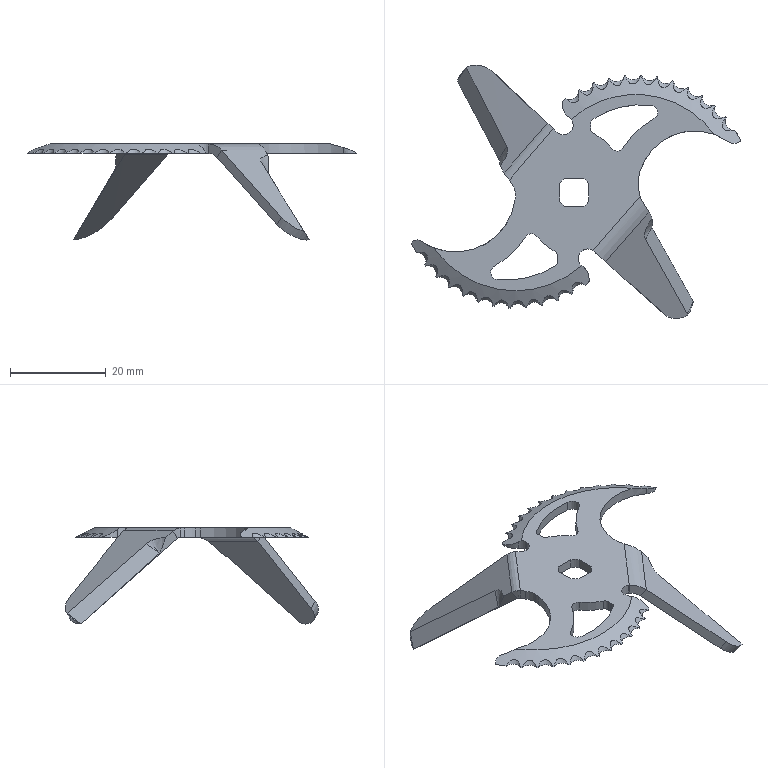Part | SolidWorks | features 3DProfileFeature 12, SweepCut 5, ICE 4, CirPattern 2, SM3dBend 2, Cut 1, FlatPattern 1, SMBaseFlange 1, SheetMetal 1 | 1 solid | 123 faces | box 68.715 x 52.833 x 20.056 mm | volume 2844 mm3 | cylinder 54 | spline 47 | plane 22 | commonest cylinder face diameters 48.461 x13 2 x6 3 x6 7 x5 12 x3 4.002 x2